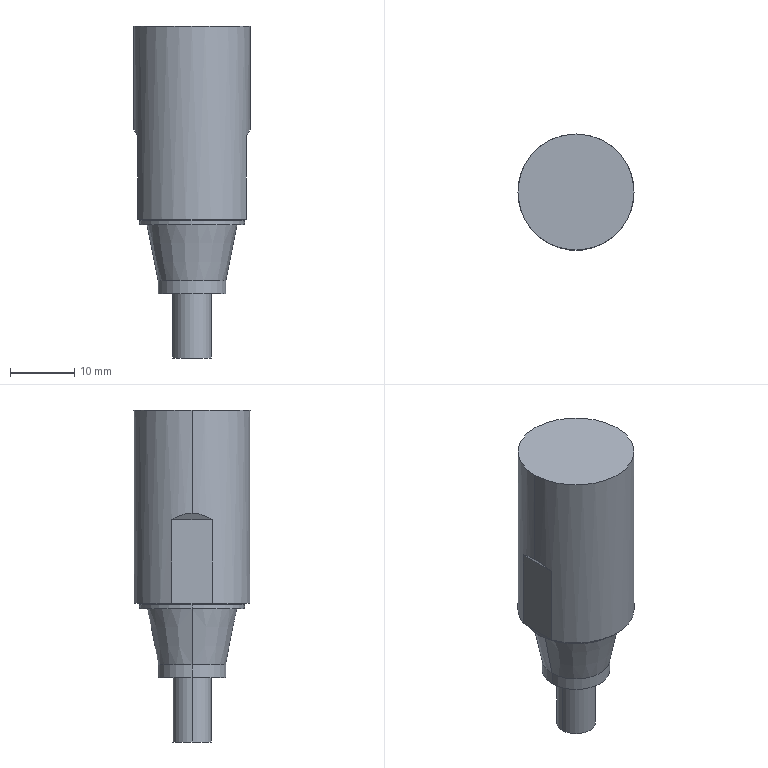Part | STEP file | E2EW-X7D118-M1TGJ0.3M-Part-1 | 1 solid | 22 faces | box 18 x 18 x 51.5 mm | volume 9224 mm3 | cylinder 10 | plane 10 | cone 2 | commonest cylinder face diameters 6 x2 10.5 x2 15.9 x2 16.3 x2 18 x2